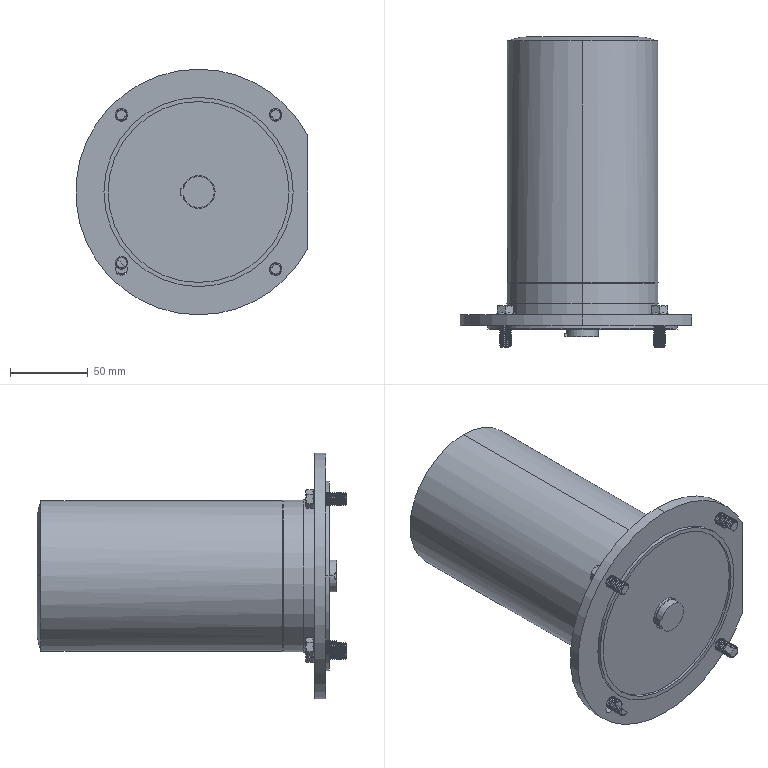Part | SolidWorks | features BaseBody 1 | 1 solid | 1407 faces | box 148.911 x 198.889 x 157.6 mm | volume 1453684 mm3 | cone 467 | torus 435 | plane 294 | cylinder 211 | commonest cylinder face diameters 8 x161 78.144 x17 7.92 x9 135 x4 157.6 x3 20.064 x2